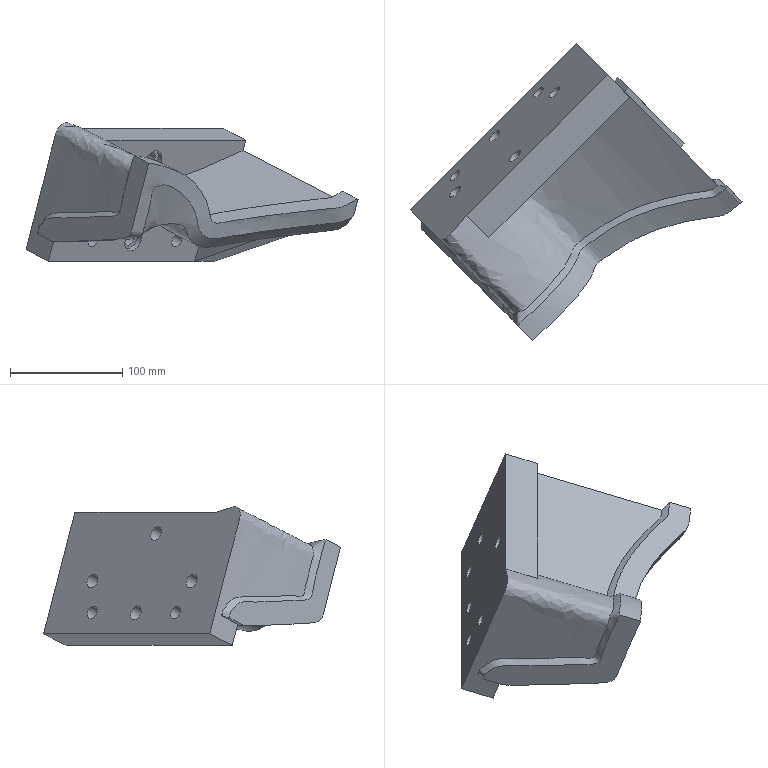Part | NX | features solid 2 | 1 solid | 38 faces | box 295.788 x 264.345 x 123.488 mm | volume 1512686 mm3 | plane 21 | cylinder 10 | spline 7 | commonest cylinder face diameters 13 x4 20 x4 12 x2